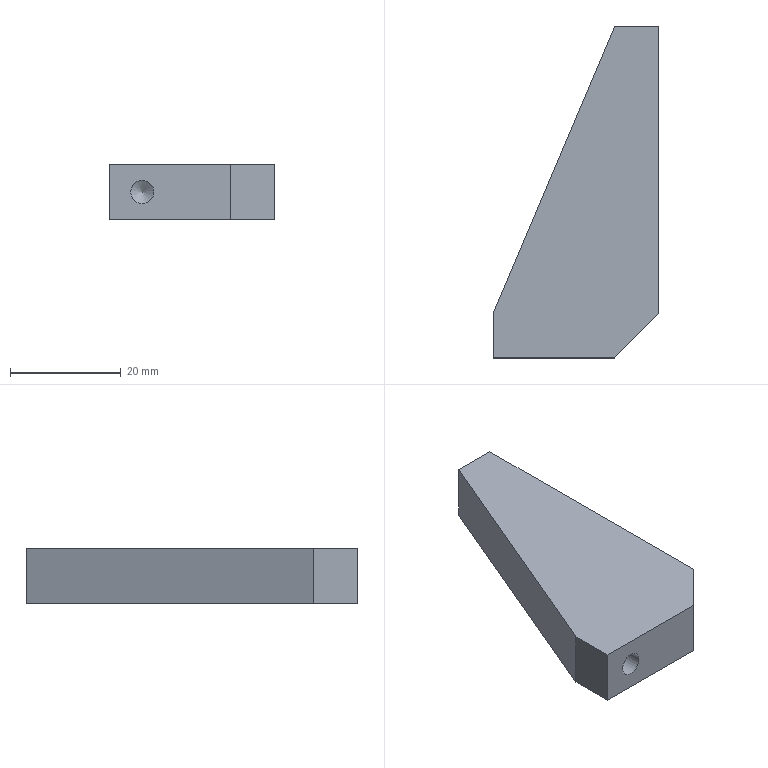Part | NX | features BREP 1 | 1 solid | 14 faces | box 30 x 60 x 10 mm | volume 11427 mm3 | plane 8 | cylinder 3 | cone 3 | commonest cylinder face diameters 4.2 x3
STEP:
#1=CARTESIAN_POINT('',(-30.,8.,0.));
#2=VERTEX_POINT('',#1);
#3=CARTESIAN_POINT('',(-30.,0.,0.));
#4=VERTEX_POINT('',#3);
#5=CARTESIAN_POINT('',(-30.,0.,0.));
#6=DIRECTION('',(0.,-1.,0.));
#7=VECTOR('',#6,1000.);
#8=LINE('',#5,#7);
#9=EDGE_CURVE('',#2,#4,#8,.T.);
#10=ORIENTED_EDGE('',*,*,#9,.F.);
#11=CARTESIAN_POINT('',(-8.,60.,0.));
#12=VERTEX_POINT('',#11);
#13=CARTESIAN_POINT('',(-8.,60.,0.));
#14=DIRECTION('',(-0.3896,-0.921,0.));
#15=VECTOR('',#14,1000.);
#16=LINE('',#13,#15);
#17=EDGE_CURVE('',#12,#2,#16,.T.);
#18=ORIENTED_EDGE('',*,*,#17,.F.);
#19=CARTESIAN_POINT('',(0.,60.,0.));
#20=VERTEX_POINT('',#19);
#21=CARTESIAN_POINT('',(0.,60.,0.));
#22=DIRECTION('',(-1.,0.,0.));
#23=VECTOR('',#22,1000.);
#24=LINE('',#21,#23);
#25=EDGE_CURVE('',#20,#12,#24,.T.);
#26=ORIENTED_EDGE('',*,*,#25,.F.);
#27=CARTESIAN_POINT('',(0.,8.,0.));
#28=VERTEX_POINT('',#27);
#29=CARTESIAN_POINT('',(0.,0.,0.));
#30=DIRECTION('',(0.,1.,0.));
#31=VECTOR('',#30,1000.);
#32=LINE('',#29,#31);
#33=EDGE_CURVE('',#28,#20,#32,.T.);
#34=ORIENTED_EDGE('',*,*,#33,.F.);
#35=CARTESIAN_POINT('',(-8.,0.,0.));
#36=VERTEX_POINT('',#35);
#37=CARTESIAN_POINT('',(-8.,0.,0.));
#38=DIRECTION('',(0.7071,0.7071,0.));
#39=VECTOR('',#38,1000.);
#40=LINE('',#37,#39);
#41=EDGE_CURVE('',#36,#28,#40,.T.);
#42=ORIENTED_EDGE('',*,*,#41,.F.);
#43=CARTESIAN_POINT('',(0.,0.,0.));
#44=DIRECTION('',(1.,0.,0.));
#45=VECTOR('',#44,1000.);
#46=LINE('',#43,#45);
#47=EDGE_CURVE('',#4,#36,#46,.T.);
#48=ORIENTED_EDGE('',*,*,#47,.F.);
#49=EDGE_LOOP('',(#10,#18,#26,#34,#42,#48));
#50=FACE_BOUND('',#49,.T.);
#51=CARTESIAN_POINT('',(0.,0.,0.));
#52=DIRECTION('',(0.,0.,1.));
#53=DIRECTION('',(-1.,0.,0.));
#54=AXIS2_PLACEMENT_3D('',#51,#52,#53);
#55=PLANE('',#54);
#56=ADVANCED_FACE('',(#50),#55,.F.);
#57=CARTESIAN_POINT('',(-8.,0.,10.));
#58=VERTEX_POINT('',#57);
#59=CARTESIAN_POINT('',(-8.,0.,10.));
#60=DIRECTION('',(0.,0.,-1.));
#61=VECTOR('',#60,1000.);
#62=LINE('',#59,#61);
#63=EDGE_CURVE('',#58,#36,#62,.T.);
#64=ORIENTED_EDGE('',*,*,#63,.F.);
#65=CARTESIAN_POINT('',(-30.,0.,10.));
#66=VERTEX_POINT('',#65);
#67=CARTESIAN_POINT('',(-30.,0.,10.));
#68=DIRECTION('',(1.,0.,0.));
#69=VECTOR('',#68,1000.);
#70=LINE('',#67,#69);
#71=EDGE_CURVE('',#66,#58,#70,.T.);
#72=ORIENTED_EDGE('',*,*,#71,.F.);
#73=CARTESIAN_POINT('',(-30.,0.,10.));
#74=DIRECTION('',(0.,0.,1.));
#75=VECTOR('',#74,1000.);
#76=LINE('',#73,#75);
#77=EDGE_CURVE('',#4,#66,#76,.T.);
#78=ORIENTED_EDGE('',*,*,#77,.F.);
#79=ORIENTED_EDGE('',*,*,#47,.T.);
#80=EDGE_LOOP('',(#64,#72,#78,#79));
#81=FACE_BOUND('',#80,.T.);
#82=CARTESIAN_POINT('',(-24.,0.,2.9));
#83=VERTEX_POINT('',#82);
#84=CARTESIAN_POINT('',(-24.,0.,5.));
#85=DIRECTION('',(0.,-1.,0.));
#86=DIRECTION('',(0.,0.,-1.));
#87=AXIS2_PLACEMENT_3D('',#84,#85,#86);
#88=CIRCLE('',#87,2.1);
#89=EDGE_CURVE('',#83,#83,#88,.T.);
#90=ORIENTED_EDGE('',*,*,#89,.F.);
#91=EDGE_LOOP('',(#90));
#92=FACE_BOUND('',#91,.T.);
#93=CARTESIAN_POINT('',(-30.,0.,10.));
#94=DIRECTION('',(0.,1.,0.));
#95=DIRECTION('',(0.,0.,-1.));
#96=AXIS2_PLACEMENT_3D('',#93,#94,#95);
#97=PLANE('',#96);
#98=ADVANCED_FACE('',(#81,#92),#97,.F.);
#99=ORIENTED_EDGE('',*,*,#77,.T.);
#100=CARTESIAN_POINT('',(-30.,8.,10.));
#101=VERTEX_POINT('',#100);
#102=CARTESIAN_POINT('',(-30.,8.,10.));
#103=DIRECTION('',(0.,-1.,0.));
#104=VECTOR('',#103,1000.);
#105=LINE('',#102,#104);
#106=EDGE_CURVE('',#101,#66,#105,.T.);
#107=ORIENTED_EDGE('',*,*,#106,.F.);
#108=CARTESIAN_POINT('',(-30.,8.,10.));
#109=DIRECTION('',(0.,0.,1.));
#110=VECTOR('',#109,1000.);
#111=LINE('',#108,#110);
#112=EDGE_CURVE('',#2,#101,#111,.T.);
#113=ORIENTED_EDGE('',*,*,#112,.F.);
#114=ORIENTED_EDGE('',*,*,#9,.T.);
#115=EDGE_LOOP('',(#99,#107,#113,#114));
#116=FACE_BOUND('',#115,.T.);
#117=CARTESIAN_POINT('',(-30.,8.,10.));
#118=DIRECTION('',(1.,0.,0.));
#119=DIRECTION('',(0.,0.,1.));
#120=AXIS2_PLACEMENT_3D('',#117,#118,#119);
#121=PLANE('',#120);
#122=ADVANCED_FACE('',(#116),#121,.F.);
#123=ORIENTED_EDGE('',*,*,#112,.T.);
#124=CARTESIAN_POINT('',(-8.,60.,10.));
#125=VERTEX_POINT('',#124);
#126=CARTESIAN_POINT('',(-8.,60.,10.));
#127=DIRECTION('',(-0.3896,-0.921,0.));
#128=VECTOR('',#127,1000.);
#129=LINE('',#126,#128);
#130=EDGE_CURVE('',#125,#101,#129,.T.);
#131=ORIENTED_EDGE('',*,*,#130,.F.);
#132=CARTESIAN_POINT('',(-8.,60.,10.));
#133=DIRECTION('',(0.,0.,1.));
#134=VECTOR('',#133,1000.);
#135=LINE('',#132,#134);
#136=EDGE_CURVE('',#12,#125,#135,.T.);
#137=ORIENTED_EDGE('',*,*,#136,.F.);
#138=ORIENTED_EDGE('',*,*,#17,.T.);
#139=EDGE_LOOP('',(#123,#131,#137,#138));
#140=FACE_BOUND('',#139,.T.);
#141=CARTESIAN_POINT('',(-8.,60.,10.));
#142=DIRECTION('',(0.921,-0.3896,0.));
#143=DIRECTION('',(-0.3896,-0.921,0.));
#144=AXIS2_PLACEMENT_3D('',#141,#142,#143);
#145=PLANE('',#144);
#146=ADVANCED_FACE('',(#140),#145,.F.);
#147=ORIENTED_EDGE('',*,*,#136,.T.);
#148=CARTESIAN_POINT('',(0.,60.,10.));
#149=VERTEX_POINT('',#148);
#150=CARTESIAN_POINT('',(0.,60.,10.));
#151=DIRECTION('',(-1.,0.,0.));
#152=VECTOR('',#151,1000.);
#153=LINE('',#150,#152);
#154=EDGE_CURVE('',#149,#125,#153,.T.);
#155=ORIENTED_EDGE('',*,*,#154,.F.);
#156=CARTESIAN_POINT('',(0.,60.,10.));
#157=DIRECTION('',(0.,0.,1.));
#158=VECTOR('',#157,1000.);
#159=LINE('',#156,#158);
#160=EDGE_CURVE('',#20,#149,#159,.T.);
#161=ORIENTED_EDGE('',*,*,#160,.F.);
#162=ORIENTED_EDGE('',*,*,#25,.T.);
#163=EDGE_LOOP('',(#147,#155,#161,#162));
#164=FACE_BOUND('',#163,.T.);
#165=CARTESIAN_POINT('',(0.,60.,10.));
#166=DIRECTION('',(0.,-1.,0.));
#167=DIRECTION('',(0.,0.,1.));
#168=AXIS2_PLACEMENT_3D('',#165,#166,#167);
#169=PLANE('',#168);
#170=ADVANCED_FACE('',(#164),#169,.F.);
#171=ORIENTED_EDGE('',*,*,#160,.T.);
#172=CARTESIAN_POINT('',(0.,8.,10.));
#173=VERTEX_POINT('',#172);
#174=CARTESIAN_POINT('',(0.,8.,10.));
#175=DIRECTION('',(0.,1.,0.));
#176=VECTOR('',#175,1000.);
#177=LINE('',#174,#176);
#178=EDGE_CURVE('',#173,#149,#177,.T.);
#179=ORIENTED_EDGE('',*,*,#178,.F.);
#180=CARTESIAN_POINT('',(0.,8.,10.));
#181=DIRECTION('',(0.,0.,1.));
#182=VECTOR('',#181,1000.);
#183=LINE('',#180,#182);
#184=EDGE_CURVE('',#28,#173,#183,.T.);
#185=ORIENTED_EDGE('',*,*,#184,.F.);
#186=ORIENTED_EDGE('',*,*,#33,.T.);
#187=EDGE_LOOP('',(#171,#179,#185,#186));
#188=FACE_BOUND('',#187,.T.);
#189=CARTESIAN_POINT('',(0.,45.,2.9));
#190=VERTEX_POINT('',#189);
#191=CARTESIAN_POINT('',(0.,45.,5.));
#192=DIRECTION('',(1.,0.,0.));
#193=DIRECTION('',(0.,0.,-1.));
#194=AXIS2_PLACEMENT_3D('',#191,#192,#193);
#195=CIRCLE('',#194,2.1);
#196=EDGE_CURVE('',#190,#190,#195,.T.);
#197=ORIENTED_EDGE('',*,*,#196,.F.);
#198=EDGE_LOOP('',(#197));
#199=FACE_BOUND('',#198,.T.);
#200=CARTESIAN_POINT('',(0.,18.,2.9));
#201=VERTEX_POINT('',#200);
#202=CARTESIAN_POINT('',(0.,18.,5.));
#203=DIRECTION('',(1.,0.,0.));
#204=DIRECTION('',(0.,0.,-1.));
#205=AXIS2_PLACEMENT_3D('',#202,#203,#204);
#206=CIRCLE('',#205,2.1);
#207=EDGE_CURVE('',#201,#201,#206,.T.);
#208=ORIENTED_EDGE('',*,*,#207,.F.);
#209=EDGE_LOOP('',(#208));
#210=FACE_BOUND('',#209,.T.);
#211=CARTESIAN_POINT('',(0.,8.,10.));
#212=DIRECTION('',(-1.,0.,0.));
#213=DIRECTION('',(0.,0.,-1.));
#214=AXIS2_PLACEMENT_3D('',#211,#212,#213);
#215=PLANE('',#214);
#216=ADVANCED_FACE('',(#188,#199,#210),#215,.F.);
#217=ORIENTED_EDGE('',*,*,#184,.T.);
#218=CARTESIAN_POINT('',(-8.,0.,10.));
#219=DIRECTION('',(0.7071,0.7071,0.));
#220=VECTOR('',#219,1000.);
#221=LINE('',#218,#220);
#222=EDGE_CURVE('',#58,#173,#221,.T.);
#223=ORIENTED_EDGE('',*,*,#222,.F.);
#224=ORIENTED_EDGE('',*,*,#63,.T.);
#225=ORIENTED_EDGE('',*,*,#41,.T.);
#226=EDGE_LOOP('',(#217,#223,#224,#225));
#227=FACE_BOUND('',#226,.T.);
#228=CARTESIAN_POINT('',(-8.,0.,10.));
#229=DIRECTION('',(-0.7071,0.7071,0.));
#230=DIRECTION('',(0.7071,0.7071,0.));
#231=AXIS2_PLACEMENT_3D('',#228,#229,#230);
#232=PLANE('',#231);
#233=ADVANCED_FACE('',(#227),#232,.F.);
#234=ORIENTED_EDGE('',*,*,#130,.T.);
#235=ORIENTED_EDGE('',*,*,#106,.T.);
#236=ORIENTED_EDGE('',*,*,#71,.T.);
#237=ORIENTED_EDGE('',*,*,#222,.T.);
#238=ORIENTED_EDGE('',*,*,#178,.T.);
#239=ORIENTED_EDGE('',*,*,#154,.T.);
#240=EDGE_LOOP('',(#234,#235,#236,#237,#238,#239));
#241=FACE_BOUND('',#240,.T.);
#242=CARTESIAN_POINT('',(0.,0.,10.));
#243=DIRECTION('',(0.,0.,1.));
#244=DIRECTION('',(-1.,0.,0.));
#245=AXIS2_PLACEMENT_3D('',#242,#243,#244);
#246=PLANE('',#245);
#247=ADVANCED_FACE('',(#241),#246,.T.);
#248=CARTESIAN_POINT('',(-24.,12.4,2.9));
#249=VERTEX_POINT('',#248);
#250=CARTESIAN_POINT('',(-24.,12.4,5.));
#251=DIRECTION('',(0.,-1.,0.));
#252=DIRECTION('',(0.,0.,-1.));
#253=AXIS2_PLACEMENT_3D('',#250,#251,#252);
#254=CIRCLE('',#253,2.1);
#255=EDGE_CURVE('',#249,#249,#254,.T.);
#256=ORIENTED_EDGE('',*,*,#255,.F.);
#257=EDGE_LOOP('',(#256));
#258=FACE_BOUND('',#257,.T.);
#259=ORIENTED_EDGE('',*,*,#89,.T.);
#260=EDGE_LOOP('',(#259));
#261=FACE_BOUND('',#260,.T.);
#262=CARTESIAN_POINT('',(-24.,0.,5.));
#263=DIRECTION('',(0.,-1.,0.));
#264=DIRECTION('',(0.,0.,1.));
#265=AXIS2_PLACEMENT_3D('',#262,#263,#264);
#266=CYLINDRICAL_SURFACE('',#265,2.1);
#267=ADVANCED_FACE('',(#258,#261),#266,.F.);
#268=CARTESIAN_POINT('',(-12.4,45.,2.9));
#269=VERTEX_POINT('',#268);
#270=CARTESIAN_POINT('',(-12.4,45.,5.));
#271=DIRECTION('',(1.,0.,0.));
#272=DIRECTION('',(0.,0.,-1.));
#273=AXIS2_PLACEMENT_3D('',#270,#271,#272);
#274=CIRCLE('',#273,2.1);
#275=EDGE_CURVE('',#269,#269,#274,.T.);
#276=ORIENTED_EDGE('',*,*,#275,.F.);
#277=EDGE_LOOP('',(#276));
#278=FACE_BOUND('',#277,.T.);
#279=ORIENTED_EDGE('',*,*,#196,.T.);
#280=EDGE_LOOP('',(#279));
#281=FACE_BOUND('',#280,.T.);
#282=CARTESIAN_POINT('',(0.,45.,5.));
#283=DIRECTION('',(1.,0.,0.));
#284=DIRECTION('',(0.,0.,1.));
#285=AXIS2_PLACEMENT_3D('',#282,#283,#284);
#286=CYLINDRICAL_SURFACE('',#285,2.1);
#287=ADVANCED_FACE('',(#278,#281),#286,.F.);
#288=CARTESIAN_POINT('',(-12.4,18.,2.9));
#289=VERTEX_POINT('',#288);
#290=CARTESIAN_POINT('',(-12.4,18.,5.));
#291=DIRECTION('',(1.,0.,0.));
#292=DIRECTION('',(0.,0.,-1.));
#293=AXIS2_PLACEMENT_3D('',#290,#291,#292);
#294=CIRCLE('',#293,2.1);
#295=EDGE_CURVE('',#289,#289,#294,.T.);
#296=ORIENTED_EDGE('',*,*,#295,.F.);
#297=EDGE_LOOP('',(#296));
#298=FACE_BOUND('',#297,.T.);
#299=ORIENTED_EDGE('',*,*,#207,.T.);
#300=EDGE_LOOP('',(#299));
#301=FACE_BOUND('',#300,.T.);
#302=CARTESIAN_POINT('',(0.,18.,5.));
#303=DIRECTION('',(1.,0.,0.));
#304=DIRECTION('',(0.,0.,1.));
#305=AXIS2_PLACEMENT_3D('',#302,#303,#304);
#306=CYLINDRICAL_SURFACE('',#305,2.1);
#307=ADVANCED_FACE('',(#298,#301),#306,.F.);
#308=CARTESIAN_POINT('',(-24.,13.662,5.));
#309=VERTEX_POINT('',#308);
#310=VERTEX_LOOP('',#309);
#311=FACE_BOUND('',#310,.T.);
#312=ORIENTED_EDGE('',*,*,#255,.T.);
#313=EDGE_LOOP('',(#312));
#314=FACE_BOUND('',#313,.T.);
#315=CARTESIAN_POINT('',(-24.,12.4,5.));
#316=DIRECTION('',(0.,-1.,0.));
#317=DIRECTION('',(0.,0.,1.));
#318=AXIS2_PLACEMENT_3D('',#315,#316,#317);
#319=CONICAL_SURFACE('',#318,2.1,1.03);
#320=ADVANCED_FACE('',(#311,#314),#319,.F.);
#321=CARTESIAN_POINT('',(-13.662,45.,5.));
#322=VERTEX_POINT('',#321);
#323=VERTEX_LOOP('',#322);
#324=FACE_BOUND('',#323,.T.);
#325=ORIENTED_EDGE('',*,*,#275,.T.);
#326=EDGE_LOOP('',(#325));
#327=FACE_BOUND('',#326,.T.);
#328=CARTESIAN_POINT('',(-12.4,45.,5.));
#329=DIRECTION('',(1.,0.,0.));
#330=DIRECTION('',(0.,0.,1.));
#331=AXIS2_PLACEMENT_3D('',#328,#329,#330);
#332=CONICAL_SURFACE('',#331,2.1,1.03);
#333=ADVANCED_FACE('',(#324,#327),#332,.F.);
#334=CARTESIAN_POINT('',(-13.662,18.,5.));
#335=VERTEX_POINT('',#334);
#336=VERTEX_LOOP('',#335);
#337=FACE_BOUND('',#336,.T.);
#338=ORIENTED_EDGE('',*,*,#295,.T.);
#339=EDGE_LOOP('',(#338));
#340=FACE_BOUND('',#339,.T.);
#341=CARTESIAN_POINT('',(-12.4,18.,5.));
#342=DIRECTION('',(1.,0.,0.));
#343=DIRECTION('',(0.,0.,1.));
#344=AXIS2_PLACEMENT_3D('',#341,#342,#343);
#345=CONICAL_SURFACE('',#344,2.1,1.03);
#346=ADVANCED_FACE('',(#337,#340),#345,.F.);
#347=CLOSED_SHELL('',(#56,#98,#122,#146,#170,#216,#233,#247,#267,#287,#307,#320,#333,#346));
#348=MANIFOLD_SOLID_BREP('',#347);
#349=(LENGTH_UNIT()NAMED_UNIT(*)SI_UNIT(.MILLI.,.METRE.));
#350=UNCERTAINTY_MEASURE_WITH_UNIT(LENGTH_MEASURE(0.00001),#349,'','');
#351=(NAMED_UNIT(*)PLANE_ANGLE_UNIT()SI_UNIT($,.RADIAN.));
#352=(NAMED_UNIT(*)SI_UNIT($,.STERADIAN.)SOLID_ANGLE_UNIT());
#353=(GEOMETRIC_REPRESENTATION_CONTEXT(3)GLOBAL_UNCERTAINTY_ASSIGNED_CONTEXT((#350))GLOBAL_UNIT_ASSIGNED_CONTEXT((#349,#351,#352))REPRESENTATION_CONTEXT('',''));
#354=ADVANCED_BREP_SHAPE_REPRESENTATION('',(#348),#353);